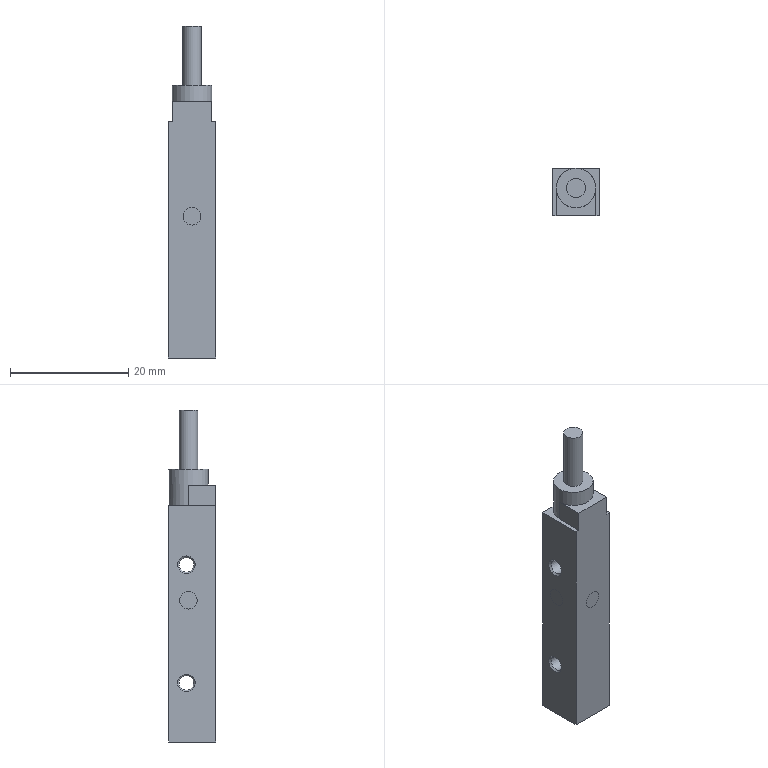Part | NX | features BREP 1 | 1 solid | 34 faces | box 8 x 8.1 x 56.2 mm | volume 2831 mm3 | plane 19 | cylinder 11 | cone 4 | commonest cylinder face diameters 3 x4 2.459 x2 3.2 x2 5.8 x1 6.7 x1 7 x1
STEP:
#1=CARTESIAN_POINT('',(0.,-4.65,-21.));
#2=VERTEX_POINT('',#1);
#3=CARTESIAN_POINT('',(0.,-4.65,-19.5));
#4=DIRECTION('',(0.,1.,0.));
#5=DIRECTION('',(0.,0.,-1.));
#6=AXIS2_PLACEMENT_3D('',#3,#4,#5);
#7=CIRCLE('',#6,1.5);
#8=EDGE_CURVE('',#2,#2,#7,.T.);
#9=ORIENTED_EDGE('',*,*,#8,.F.);
#10=EDGE_LOOP('',(#9));
#11=FACE_BOUND('',#10,.T.);
#12=CARTESIAN_POINT('',(0.,-4.649,-18.));
#13=VERTEX_POINT('',#12);
#14=CARTESIAN_POINT('',(0.,-4.649,-19.5));
#15=DIRECTION('',(0.,1.,0.));
#16=DIRECTION('',(0.,0.,1.));
#17=AXIS2_PLACEMENT_3D('',#14,#15,#16);
#18=CIRCLE('',#17,1.5);
#19=EDGE_CURVE('',#13,#13,#18,.T.);
#20=ORIENTED_EDGE('',*,*,#19,.T.);
#21=EDGE_LOOP('',(#20));
#22=FACE_BOUND('',#21,.T.);
#23=CARTESIAN_POINT('',(0.,5.,-19.5));
#24=DIRECTION('',(0.,-1.,0.));
#25=DIRECTION('',(0.,0.,1.));
#26=AXIS2_PLACEMENT_3D('',#23,#24,#25);
#27=CYLINDRICAL_SURFACE('',#26,1.5);
#28=ADVANCED_FACE('',(#11,#22),#27,.F.);
#29=CARTESIAN_POINT('',(-4.,0.,-18.));
#30=VERTEX_POINT('',#29);
#31=CARTESIAN_POINT('',(-4.,0.,-19.5));
#32=DIRECTION('',(1.,0.,0.));
#33=DIRECTION('',(0.,0.,1.));
#34=AXIS2_PLACEMENT_3D('',#31,#32,#33);
#35=CIRCLE('',#34,1.5);
#36=EDGE_CURVE('',#30,#30,#35,.T.);
#37=ORIENTED_EDGE('',*,*,#36,.F.);
#38=EDGE_LOOP('',(#37));
#39=FACE_BOUND('',#38,.T.);
#40=CARTESIAN_POINT('',(-3.999,0.,-21.));
#41=VERTEX_POINT('',#40);
#42=CARTESIAN_POINT('',(-3.999,0.,-19.5));
#43=DIRECTION('',(1.,0.,0.));
#44=DIRECTION('',(0.,0.,-1.));
#45=AXIS2_PLACEMENT_3D('',#42,#43,#44);
#46=CIRCLE('',#45,1.5);
#47=EDGE_CURVE('',#41,#41,#46,.T.);
#48=ORIENTED_EDGE('',*,*,#47,.T.);
#49=EDGE_LOOP('',(#48));
#50=FACE_BOUND('',#49,.T.);
#51=CARTESIAN_POINT('',(5.,0.,-19.5));
#52=DIRECTION('',(-1.,0.,0.));
#53=DIRECTION('',(0.,0.,-1.));
#54=AXIS2_PLACEMENT_3D('',#51,#52,#53);
#55=CYLINDRICAL_SURFACE('',#54,1.5);
#56=ADVANCED_FACE('',(#39,#50),#55,.F.);
#57=CARTESIAN_POINT('',(0.,3.349,-18.));
#58=VERTEX_POINT('',#57);
#59=CARTESIAN_POINT('',(0.,3.349,-19.5));
#60=DIRECTION('',(0.,1.,0.));
#61=DIRECTION('',(0.,0.,1.));
#62=AXIS2_PLACEMENT_3D('',#59,#60,#61);
#63=CIRCLE('',#62,1.5);
#64=EDGE_CURVE('',#58,#58,#63,.T.);
#65=ORIENTED_EDGE('',*,*,#64,.F.);
#66=EDGE_LOOP('',(#65));
#67=FACE_BOUND('',#66,.T.);
#68=CARTESIAN_POINT('',(0.,3.35,-18.));
#69=VERTEX_POINT('',#68);
#70=CARTESIAN_POINT('',(0.,3.35,-19.5));
#71=DIRECTION('',(0.,-1.,0.));
#72=DIRECTION('',(0.,0.,1.));
#73=AXIS2_PLACEMENT_3D('',#70,#71,#72);
#74=CIRCLE('',#73,1.5);
#75=EDGE_CURVE('',#69,#69,#74,.T.);
#76=ORIENTED_EDGE('',*,*,#75,.F.);
#77=EDGE_LOOP('',(#76));
#78=FACE_BOUND('',#77,.T.);
#79=CARTESIAN_POINT('',(0.,5.,-19.5));
#80=DIRECTION('',(0.,-1.,0.));
#81=DIRECTION('',(0.,0.,1.));
#82=AXIS2_PLACEMENT_3D('',#79,#80,#81);
#83=CYLINDRICAL_SURFACE('',#82,1.5);
#84=ADVANCED_FACE('',(#67,#78),#83,.F.);
#85=CARTESIAN_POINT('',(3.999,0.,-21.));
#86=VERTEX_POINT('',#85);
#87=CARTESIAN_POINT('',(3.999,0.,-19.5));
#88=DIRECTION('',(1.,0.,0.));
#89=DIRECTION('',(0.,0.,-1.));
#90=AXIS2_PLACEMENT_3D('',#87,#88,#89);
#91=CIRCLE('',#90,1.5);
#92=EDGE_CURVE('',#86,#86,#91,.T.);
#93=ORIENTED_EDGE('',*,*,#92,.F.);
#94=EDGE_LOOP('',(#93));
#95=FACE_BOUND('',#94,.T.);
#96=CARTESIAN_POINT('',(4.,0.,-21.));
#97=VERTEX_POINT('',#96);
#98=CARTESIAN_POINT('',(4.,0.,-19.5));
#99=DIRECTION('',(-1.,0.,0.));
#100=DIRECTION('',(0.,0.,-1.));
#101=AXIS2_PLACEMENT_3D('',#98,#99,#100);
#102=CIRCLE('',#101,1.5);
#103=EDGE_CURVE('',#97,#97,#102,.T.);
#104=ORIENTED_EDGE('',*,*,#103,.F.);
#105=EDGE_LOOP('',(#104));
#106=FACE_BOUND('',#105,.T.);
#107=CARTESIAN_POINT('',(5.,0.,-19.5));
#108=DIRECTION('',(-1.,0.,0.));
#109=DIRECTION('',(0.,0.,-1.));
#110=AXIS2_PLACEMENT_3D('',#107,#108,#109);
#111=CYLINDRICAL_SURFACE('',#110,1.5);
#112=ADVANCED_FACE('',(#95,#106),#111,.F.);
#113=CARTESIAN_POINT('',(3.35,0.,2.7));
#114=VERTEX_POINT('',#113);
#115=CARTESIAN_POINT('',(0.,0.,2.7));
#116=DIRECTION('',(0.,0.,1.));
#117=DIRECTION('',(1.,0.,0.));
#118=AXIS2_PLACEMENT_3D('',#115,#116,#117);
#119=CIRCLE('',#118,3.35);
#120=EDGE_CURVE('',#114,#114,#119,.T.);
#121=ORIENTED_EDGE('',*,*,#120,.F.);
#122=EDGE_LOOP('',(#121));
#123=FACE_BOUND('',#122,.T.);
#124=CARTESIAN_POINT('',(-3.35,0.,0.));
#125=VERTEX_POINT('',#124);
#126=CARTESIAN_POINT('',(3.35,0.,0.));
#127=VERTEX_POINT('',#126);
#128=CARTESIAN_POINT('',(0.,0.,0.));
#129=DIRECTION('',(0.,0.,1.));
#130=DIRECTION('',(1.,0.,0.));
#131=AXIS2_PLACEMENT_3D('',#128,#129,#130);
#132=CIRCLE('',#131,3.35);
#133=EDGE_CURVE('',#125,#127,#132,.T.);
#134=ORIENTED_EDGE('',*,*,#133,.T.);
#135=CARTESIAN_POINT('',(3.35,0.,-3.5));
#136=VERTEX_POINT('',#135);
#137=CARTESIAN_POINT('',(3.35,0.,-3.5));
#138=DIRECTION('',(0.,0.,1.));
#139=VECTOR('',#138,1000.);
#140=LINE('',#137,#139);
#141=EDGE_CURVE('',#136,#127,#140,.T.);
#142=ORIENTED_EDGE('',*,*,#141,.F.);
#143=CARTESIAN_POINT('',(0.,3.35,-3.5));
#144=VERTEX_POINT('',#143);
#145=CARTESIAN_POINT('',(0.,0.,-3.5));
#146=DIRECTION('',(0.,0.,1.));
#147=DIRECTION('',(1.,0.,0.));
#148=AXIS2_PLACEMENT_3D('',#145,#146,#147);
#149=CIRCLE('',#148,3.35);
#150=EDGE_CURVE('',#136,#144,#149,.T.);
#151=ORIENTED_EDGE('',*,*,#150,.T.);
#152=CARTESIAN_POINT('',(-3.35,0.,-3.5));
#153=VERTEX_POINT('',#152);
#154=CARTESIAN_POINT('',(0.,0.,-3.5));
#155=DIRECTION('',(0.,0.,1.));
#156=DIRECTION('',(1.,0.,0.));
#157=AXIS2_PLACEMENT_3D('',#154,#155,#156);
#158=CIRCLE('',#157,3.35);
#159=EDGE_CURVE('',#144,#153,#158,.T.);
#160=ORIENTED_EDGE('',*,*,#159,.T.);
#161=CARTESIAN_POINT('',(-3.35,0.,-3.5));
#162=DIRECTION('',(0.,0.,1.));
#163=VECTOR('',#162,1000.);
#164=LINE('',#161,#163);
#165=EDGE_CURVE('',#153,#125,#164,.T.);
#166=ORIENTED_EDGE('',*,*,#165,.T.);
#167=EDGE_LOOP('',(#134,#142,#151,#160,#166));
#168=FACE_BOUND('',#167,.T.);
#169=CARTESIAN_POINT('',(0.,0.,2.7));
#170=DIRECTION('',(0.,0.,-1.));
#171=DIRECTION('',(1.,0.,0.));
#172=AXIS2_PLACEMENT_3D('',#169,#170,#171);
#173=CYLINDRICAL_SURFACE('',#172,3.35);
#174=ADVANCED_FACE('',(#123,#168),#173,.T.);
#175=CARTESIAN_POINT('',(1.6,0.,2.7));
#176=VERTEX_POINT('',#175);
#177=CARTESIAN_POINT('',(0.,0.,2.7));
#178=DIRECTION('',(0.,0.,-1.));
#179=DIRECTION('',(1.,0.,0.));
#180=AXIS2_PLACEMENT_3D('',#177,#178,#179);
#181=CIRCLE('',#180,1.6);
#182=EDGE_CURVE('',#176,#176,#181,.T.);
#183=ORIENTED_EDGE('',*,*,#182,.T.);
#184=EDGE_LOOP('',(#183));
#185=FACE_BOUND('',#184,.T.);
#186=ORIENTED_EDGE('',*,*,#120,.T.);
#187=EDGE_LOOP('',(#186));
#188=FACE_BOUND('',#187,.T.);
#189=CARTESIAN_POINT('',(0.,0.,2.7));
#190=DIRECTION('',(0.,0.,1.));
#191=DIRECTION('',(-1.,0.,0.));
#192=AXIS2_PLACEMENT_3D('',#189,#190,#191);
#193=PLANE('',#192);
#194=ADVANCED_FACE('',(#185,#188),#193,.T.);
#195=ORIENTED_EDGE('',*,*,#133,.F.);
#196=CARTESIAN_POINT('',(-3.35,-4.65,0.));
#197=VERTEX_POINT('',#196);
#198=CARTESIAN_POINT('',(-3.35,0.,0.));
#199=DIRECTION('',(0.,-1.,0.));
#200=VECTOR('',#199,1000.);
#201=LINE('',#198,#200);
#202=EDGE_CURVE('',#125,#197,#201,.T.);
#203=ORIENTED_EDGE('',*,*,#202,.T.);
#204=CARTESIAN_POINT('',(3.35,-4.65,0.));
#205=VERTEX_POINT('',#204);
#206=CARTESIAN_POINT('',(-3.35,-4.65,0.));
#207=DIRECTION('',(1.,0.,0.));
#208=VECTOR('',#207,1000.);
#209=LINE('',#206,#208);
#210=EDGE_CURVE('',#197,#205,#209,.T.);
#211=ORIENTED_EDGE('',*,*,#210,.T.);
#212=CARTESIAN_POINT('',(3.35,-4.65,0.));
#213=DIRECTION('',(0.,1.,0.));
#214=VECTOR('',#213,1000.);
#215=LINE('',#212,#214);
#216=EDGE_CURVE('',#205,#127,#215,.T.);
#217=ORIENTED_EDGE('',*,*,#216,.T.);
#218=EDGE_LOOP('',(#195,#203,#211,#217));
#219=FACE_BOUND('',#218,.T.);
#220=CARTESIAN_POINT('',(0.,0.,0.));
#221=DIRECTION('',(0.,0.,1.));
#222=DIRECTION('',(-1.,0.,0.));
#223=AXIS2_PLACEMENT_3D('',#220,#221,#222);
#224=PLANE('',#223);
#225=ADVANCED_FACE('',(#219),#224,.T.);
#226=ORIENTED_EDGE('',*,*,#202,.F.);
#227=ORIENTED_EDGE('',*,*,#165,.F.);
#228=CARTESIAN_POINT('',(-3.35,-4.65,-3.5));
#229=VERTEX_POINT('',#228);
#230=CARTESIAN_POINT('',(-3.35,0.,-3.5));
#231=DIRECTION('',(0.,-1.,0.));
#232=VECTOR('',#231,1000.);
#233=LINE('',#230,#232);
#234=EDGE_CURVE('',#153,#229,#233,.T.);
#235=ORIENTED_EDGE('',*,*,#234,.T.);
#236=CARTESIAN_POINT('',(-3.35,-4.65,-3.5));
#237=DIRECTION('',(0.,0.,1.));
#238=VECTOR('',#237,1000.);
#239=LINE('',#236,#238);
#240=EDGE_CURVE('',#229,#197,#239,.T.);
#241=ORIENTED_EDGE('',*,*,#240,.T.);
#242=EDGE_LOOP('',(#226,#227,#235,#241));
#243=FACE_BOUND('',#242,.T.);
#244=CARTESIAN_POINT('',(-3.35,0.,-3.5));
#245=DIRECTION('',(-1.,0.,0.));
#246=DIRECTION('',(0.,0.,-1.));
#247=AXIS2_PLACEMENT_3D('',#244,#245,#246);
#248=PLANE('',#247);
#249=ADVANCED_FACE('',(#243),#248,.T.);
#250=ORIENTED_EDGE('',*,*,#8,.T.);
#251=EDGE_LOOP('',(#250));
#252=FACE_BOUND('',#251,.T.);
#253=ORIENTED_EDGE('',*,*,#210,.F.);
#254=ORIENTED_EDGE('',*,*,#240,.F.);
#255=CARTESIAN_POINT('',(-4.,-4.65,-3.5));
#256=VERTEX_POINT('',#255);
#257=CARTESIAN_POINT('',(-4.,-4.65,-3.5));
#258=DIRECTION('',(1.,0.,0.));
#259=VECTOR('',#258,1000.);
#260=LINE('',#257,#259);
#261=EDGE_CURVE('',#256,#229,#260,.T.);
#262=ORIENTED_EDGE('',*,*,#261,.F.);
#263=CARTESIAN_POINT('',(-4.,-4.65,-43.5));
#264=VERTEX_POINT('',#263);
#265=CARTESIAN_POINT('',(-4.,-4.65,-43.5));
#266=DIRECTION('',(0.,0.,1.));
#267=VECTOR('',#266,1000.);
#268=LINE('',#265,#267);
#269=EDGE_CURVE('',#264,#256,#268,.T.);
#270=ORIENTED_EDGE('',*,*,#269,.F.);
#271=CARTESIAN_POINT('',(4.,-4.65,-43.5));
#272=VERTEX_POINT('',#271);
#273=CARTESIAN_POINT('',(-4.,-4.65,-43.5));
#274=DIRECTION('',(1.,0.,0.));
#275=VECTOR('',#274,1000.);
#276=LINE('',#273,#275);
#277=EDGE_CURVE('',#264,#272,#276,.T.);
#278=ORIENTED_EDGE('',*,*,#277,.T.);
#279=CARTESIAN_POINT('',(4.,-4.65,-3.5));
#280=VERTEX_POINT('',#279);
#281=CARTESIAN_POINT('',(4.,-4.65,-43.5));
#282=DIRECTION('',(0.,0.,1.));
#283=VECTOR('',#282,1000.);
#284=LINE('',#281,#283);
#285=EDGE_CURVE('',#272,#280,#284,.T.);
#286=ORIENTED_EDGE('',*,*,#285,.T.);
#287=CARTESIAN_POINT('',(3.35,-4.65,-3.5));
#288=VERTEX_POINT('',#287);
#289=CARTESIAN_POINT('',(-4.,-4.65,-3.5));
#290=DIRECTION('',(1.,0.,0.));
#291=VECTOR('',#290,1000.);
#292=LINE('',#289,#291);
#293=EDGE_CURVE('',#288,#280,#292,.T.);
#294=ORIENTED_EDGE('',*,*,#293,.F.);
#295=CARTESIAN_POINT('',(3.35,-4.65,-3.5));
#296=DIRECTION('',(0.,0.,1.));
#297=VECTOR('',#296,1000.);
#298=LINE('',#295,#297);
#299=EDGE_CURVE('',#288,#205,#298,.T.);
#300=ORIENTED_EDGE('',*,*,#299,.T.);
#301=EDGE_LOOP('',(#253,#254,#262,#270,#278,#286,#294,#300));
#302=FACE_BOUND('',#301,.T.);
#303=CARTESIAN_POINT('',(-3.35,-4.65,-3.5));
#304=DIRECTION('',(0.,-1.,0.));
#305=DIRECTION('',(0.,0.,1.));
#306=AXIS2_PLACEMENT_3D('',#303,#304,#305);
#307=PLANE('',#306);
#308=ADVANCED_FACE('',(#252,#302),#307,.T.);
#309=ORIENTED_EDGE('',*,*,#216,.F.);
#310=ORIENTED_EDGE('',*,*,#299,.F.);
#311=CARTESIAN_POINT('',(3.35,-4.65,-3.5));
#312=DIRECTION('',(0.,1.,0.));
#313=VECTOR('',#312,1000.);
#314=LINE('',#311,#313);
#315=EDGE_CURVE('',#288,#136,#314,.T.);
#316=ORIENTED_EDGE('',*,*,#315,.T.);
#317=ORIENTED_EDGE('',*,*,#141,.T.);
#318=EDGE_LOOP('',(#309,#310,#316,#317));
#319=FACE_BOUND('',#318,.T.);
#320=CARTESIAN_POINT('',(3.35,-4.65,-3.5));
#321=DIRECTION('',(1.,0.,0.));
#322=DIRECTION('',(0.,0.,1.));
#323=AXIS2_PLACEMENT_3D('',#320,#321,#322);
#324=PLANE('',#323);
#325=ADVANCED_FACE('',(#319),#324,.T.);
#326=ORIENTED_EDGE('',*,*,#315,.F.);
#327=ORIENTED_EDGE('',*,*,#293,.T.);
#328=CARTESIAN_POINT('',(4.,3.35,-3.5));
#329=VERTEX_POINT('',#328);
#330=CARTESIAN_POINT('',(4.,-4.65,-3.5));
#331=DIRECTION('',(0.,1.,0.));
#332=VECTOR('',#331,1000.);
#333=LINE('',#330,#332);
#334=EDGE_CURVE('',#280,#329,#333,.T.);
#335=ORIENTED_EDGE('',*,*,#334,.T.);
#336=CARTESIAN_POINT('',(4.,3.35,-3.5));
#337=DIRECTION('',(-1.,0.,0.));
#338=VECTOR('',#337,1000.);
#339=LINE('',#336,#338);
#340=EDGE_CURVE('',#329,#144,#339,.T.);
#341=ORIENTED_EDGE('',*,*,#340,.T.);
#342=ORIENTED_EDGE('',*,*,#150,.F.);
#343=EDGE_LOOP('',(#326,#327,#335,#341,#342));
#344=FACE_BOUND('',#343,.T.);
#345=CARTESIAN_POINT('',(0.,0.,-3.5));
#346=DIRECTION('',(0.,0.,1.));
#347=DIRECTION('',(-1.,0.,0.));
#348=AXIS2_PLACEMENT_3D('',#345,#346,#347);
#349=PLANE('',#348);
#350=ADVANCED_FACE('',(#344),#349,.T.);
#351=ORIENTED_EDGE('',*,*,#159,.F.);
#352=CARTESIAN_POINT('',(-4.,3.35,-3.5));
#353=VERTEX_POINT('',#352);
#354=CARTESIAN_POINT('',(4.,3.35,-3.5));
#355=DIRECTION('',(-1.,0.,0.));
#356=VECTOR('',#355,1000.);
#357=LINE('',#354,#356);
#358=EDGE_CURVE('',#144,#353,#357,.T.);
#359=ORIENTED_EDGE('',*,*,#358,.T.);
#360=CARTESIAN_POINT('',(-4.,3.35,-3.5));
#361=DIRECTION('',(0.,-1.,0.));
#362=VECTOR('',#361,1000.);
#363=LINE('',#360,#362);
#364=EDGE_CURVE('',#353,#256,#363,.T.);
#365=ORIENTED_EDGE('',*,*,#364,.T.);
#366=ORIENTED_EDGE('',*,*,#261,.T.);
#367=ORIENTED_EDGE('',*,*,#234,.F.);
#368=EDGE_LOOP('',(#351,#359,#365,#366,#367));
#369=FACE_BOUND('',#368,.T.);
#370=CARTESIAN_POINT('',(0.,0.,-3.5));
#371=DIRECTION('',(0.,0.,1.));
#372=DIRECTION('',(-1.,0.,0.));
#373=AXIS2_PLACEMENT_3D('',#370,#371,#372);
#374=PLANE('',#373);
#375=ADVANCED_FACE('',(#369),#374,.T.);
#376=ORIENTED_EDGE('',*,*,#75,.T.);
#377=EDGE_LOOP('',(#376));
#378=FACE_BOUND('',#377,.T.);
#379=CARTESIAN_POINT('',(3.5,3.35,-38.5));
#380=VERTEX_POINT('',#379);
#381=CARTESIAN_POINT('',(0.,3.35,-38.5));
#382=DIRECTION('',(0.,1.,0.));
#383=DIRECTION('',(1.,0.,0.));
#384=AXIS2_PLACEMENT_3D('',#381,#382,#383);
#385=CIRCLE('',#384,3.5);
#386=EDGE_CURVE('',#380,#380,#385,.T.);
#387=ORIENTED_EDGE('',*,*,#386,.F.);
#388=EDGE_LOOP('',(#387));
#389=FACE_BOUND('',#388,.T.);
#390=ORIENTED_EDGE('',*,*,#340,.F.);
#391=CARTESIAN_POINT('',(4.,3.35,-43.5));
#392=VERTEX_POINT('',#391);
#393=CARTESIAN_POINT('',(4.,3.35,-43.5));
#394=DIRECTION('',(0.,0.,1.));
#395=VECTOR('',#394,1000.);
#396=LINE('',#393,#395);
#397=EDGE_CURVE('',#392,#329,#396,.T.);
#398=ORIENTED_EDGE('',*,*,#397,.F.);
#399=CARTESIAN_POINT('',(-4.,3.35,-43.5));
#400=VERTEX_POINT('',#399);
#401=CARTESIAN_POINT('',(4.,3.35,-43.5));
#402=DIRECTION('',(-1.,0.,0.));
#403=VECTOR('',#402,1000.);
#404=LINE('',#401,#403);
#405=EDGE_CURVE('',#392,#400,#404,.T.);
#406=ORIENTED_EDGE('',*,*,#405,.T.);
#407=CARTESIAN_POINT('',(-4.,3.35,-43.5));
#408=DIRECTION('',(0.,0.,1.));
#409=VECTOR('',#408,1000.);
#410=LINE('',#407,#409);
#411=EDGE_CURVE('',#400,#353,#410,.T.);
#412=ORIENTED_EDGE('',*,*,#411,.T.);
#413=ORIENTED_EDGE('',*,*,#358,.F.);
#414=EDGE_LOOP('',(#390,#398,#406,#412,#413));
#415=FACE_BOUND('',#414,.T.);
#416=CARTESIAN_POINT('',(4.,3.35,-43.5));
#417=DIRECTION('',(0.,1.,0.));
#418=DIRECTION('',(0.,0.,-1.));
#419=AXIS2_PLACEMENT_3D('',#416,#417,#418);
#420=PLANE('',#419);
#421=ADVANCED_FACE('',(#378,#389,#415),#420,.T.);
#422=ORIENTED_EDGE('',*,*,#36,.T.);
#423=EDGE_LOOP('',(#422));
#424=FACE_BOUND('',#423,.T.);
#425=CARTESIAN_POINT('',(-4.,0.35,-15.));
#426=VERTEX_POINT('',#425);
#427=CARTESIAN_POINT('',(-4.,0.35,-13.5));
#428=DIRECTION('',(1.,0.,0.));
#429=DIRECTION('',(0.,0.,-1.));
#430=AXIS2_PLACEMENT_3D('',#427,#428,#429);
#431=CIRCLE('',#430,1.5);
#432=EDGE_CURVE('',#426,#426,#431,.T.);
#433=ORIENTED_EDGE('',*,*,#432,.T.);
#434=EDGE_LOOP('',(#433));
#435=FACE_BOUND('',#434,.T.);
#436=CARTESIAN_POINT('',(-4.,0.35,-35.));
#437=VERTEX_POINT('',#436);
#438=CARTESIAN_POINT('',(-4.,0.35,-33.5));
#439=DIRECTION('',(1.,0.,0.));
#440=DIRECTION('',(0.,0.,-1.));
#441=AXIS2_PLACEMENT_3D('',#438,#439,#440);
#442=CIRCLE('',#441,1.5);
#443=EDGE_CURVE('',#437,#437,#442,.T.);
#444=ORIENTED_EDGE('',*,*,#443,.T.);
#445=EDGE_LOOP('',(#444));
#446=FACE_BOUND('',#445,.T.);
#447=ORIENTED_EDGE('',*,*,#364,.F.);
#448=ORIENTED_EDGE('',*,*,#411,.F.);
#449=CARTESIAN_POINT('',(-4.,3.35,-43.5));
#450=DIRECTION('',(0.,-1.,0.));
#451=VECTOR('',#450,1000.);
#452=LINE('',#449,#451);
#453=EDGE_CURVE('',#400,#264,#452,.T.);
#454=ORIENTED_EDGE('',*,*,#453,.T.);
#455=ORIENTED_EDGE('',*,*,#269,.T.);
#456=EDGE_LOOP('',(#447,#448,#454,#455));
#457=FACE_BOUND('',#456,.T.);
#458=CARTESIAN_POINT('',(-4.,3.35,-43.5));
#459=DIRECTION('',(-1.,0.,0.));
#460=DIRECTION('',(0.,0.,-1.));
#461=AXIS2_PLACEMENT_3D('',#458,#459,#460);
#462=PLANE('',#461);
#463=ADVANCED_FACE('',(#424,#435,#446,#457),#462,.T.);
#464=ORIENTED_EDGE('',*,*,#103,.T.);
#465=EDGE_LOOP('',(#464));
#466=FACE_BOUND('',#465,.T.);
#467=CARTESIAN_POINT('',(4.,0.35,-15.));
#468=VERTEX_POINT('',#467);
#469=CARTESIAN_POINT('',(4.,0.35,-13.5));
#470=DIRECTION('',(1.,0.,0.));
#471=DIRECTION('',(0.,0.,-1.));
#472=AXIS2_PLACEMENT_3D('',#469,#470,#471);
#473=CIRCLE('',#472,1.5);
#474=EDGE_CURVE('',#468,#468,#473,.T.);
#475=ORIENTED_EDGE('',*,*,#474,.F.);
#476=EDGE_LOOP('',(#475));
#477=FACE_BOUND('',#476,.T.);
#478=CARTESIAN_POINT('',(4.,0.35,-35.));
#479=VERTEX_POINT('',#478);
#480=CARTESIAN_POINT('',(4.,0.35,-33.5));
#481=DIRECTION('',(1.,0.,0.));
#482=DIRECTION('',(0.,0.,-1.));
#483=AXIS2_PLACEMENT_3D('',#480,#481,#482);
#484=CIRCLE('',#483,1.5);
#485=EDGE_CURVE('',#479,#479,#484,.T.);
#486=ORIENTED_EDGE('',*,*,#485,.F.);
#487=EDGE_LOOP('',(#486));
#488=FACE_BOUND('',#487,.T.);
#489=ORIENTED_EDGE('',*,*,#334,.F.);
#490=ORIENTED_EDGE('',*,*,#285,.F.);
#491=CARTESIAN_POINT('',(4.,-4.65,-43.5));
#492=DIRECTION('',(0.,1.,0.));
#493=VECTOR('',#492,1000.);
#494=LINE('',#491,#493);
#495=EDGE_CURVE('',#272,#392,#494,.T.);
#496=ORIENTED_EDGE('',*,*,#495,.T.);
#497=ORIENTED_EDGE('',*,*,#397,.T.);
#498=EDGE_LOOP('',(#489,#490,#496,#497));
#499=FACE_BOUND('',#498,.T.);
#500=CARTESIAN_POINT('',(4.,-4.65,-43.5));
#501=DIRECTION('',(1.,0.,0.));
#502=DIRECTION('',(0.,0.,1.));
#503=AXIS2_PLACEMENT_3D('',#500,#501,#502);
#504=PLANE('',#503);
#505=ADVANCED_FACE('',(#466,#477,#488,#499),#504,.T.);
#506=ORIENTED_EDGE('',*,*,#405,.F.);
#507=ORIENTED_EDGE('',*,*,#495,.F.);
#508=ORIENTED_EDGE('',*,*,#277,.F.);
#509=ORIENTED_EDGE('',*,*,#453,.F.);
#510=EDGE_LOOP('',(#506,#507,#508,#509));
#511=FACE_BOUND('',#510,.T.);
#512=CARTESIAN_POINT('',(0.,0.,-43.5));
#513=DIRECTION('',(0.,0.,1.));
#514=DIRECTION('',(-1.,0.,0.));
#515=AXIS2_PLACEMENT_3D('',#512,#513,#514);
#516=PLANE('',#515);
#517=ADVANCED_FACE('',(#511),#516,.F.);
#518=CARTESIAN_POINT('',(-3.729,0.35,-34.73));
#519=VERTEX_POINT('',#518);
#520=CARTESIAN_POINT('',(-3.729,0.35,-33.5));
#521=DIRECTION('',(1.,0.,0.));
#522=DIRECTION('',(0.,0.,-1.));
#523=AXIS2_PLACEMENT_3D('',#520,#521,#522);
#524=CIRCLE('',#523,1.23);
#525=EDGE_CURVE('',#519,#519,#524,.T.);
#526=ORIENTED_EDGE('',*,*,#525,.T.);
#527=EDGE_LOOP('',(#526));
#528=FACE_BOUND('',#527,.T.);
#529=ORIENTED_EDGE('',*,*,#443,.F.);
#530=EDGE_LOOP('',(#529));
#531=FACE_BOUND('',#530,.T.);
#532=CARTESIAN_POINT('',(-4.,0.35,-33.5));
#533=DIRECTION('',(-1.,0.,0.));
#534=DIRECTION('',(0.,0.,-1.));
#535=AXIS2_PLACEMENT_3D('',#532,#533,#534);
#536=CONICAL_SURFACE('',#535,1.5,0.7854);
#537=ADVANCED_FACE('',(#528,#531),#536,.F.);
#538=CARTESIAN_POINT('',(3.729,0.35,-34.73));
#539=VERTEX_POINT('',#538);
#540=CARTESIAN_POINT('',(3.729,0.35,-33.5));
#541=DIRECTION('',(1.,0.,0.));
#542=DIRECTION('',(0.,0.,-1.));
#543=AXIS2_PLACEMENT_3D('',#540,#541,#542);
#544=CIRCLE('',#543,1.23);
#545=EDGE_CURVE('',#539,#539,#544,.T.);
#546=ORIENTED_EDGE('',*,*,#545,.T.);
#547=EDGE_LOOP('',(#546));
#548=FACE_BOUND('',#547,.T.);
#549=ORIENTED_EDGE('',*,*,#525,.F.);
#550=EDGE_LOOP('',(#549));
#551=FACE_BOUND('',#550,.T.);
#552=CARTESIAN_POINT('',(4.,0.35,-33.5));
#553=DIRECTION('',(1.,0.,0.));
#554=DIRECTION('',(0.,0.,1.));
#555=AXIS2_PLACEMENT_3D('',#552,#553,#554);
#556=CYLINDRICAL_SURFACE('',#555,1.23);
#557=ADVANCED_FACE('',(#548,#551),#556,.F.);
#558=ORIENTED_EDGE('',*,*,#485,.T.);
#559=EDGE_LOOP('',(#558));
#560=FACE_BOUND('',#559,.T.);
#561=ORIENTED_EDGE('',*,*,#545,.F.);
#562=EDGE_LOOP('',(#561));
#563=FACE_BOUND('',#562,.T.);
#564=CARTESIAN_POINT('',(3.729,0.35,-33.5));
#565=DIRECTION('',(1.,0.,0.));
#566=DIRECTION('',(0.,0.,1.));
#567=AXIS2_PLACEMENT_3D('',#564,#565,#566);
#568=CONICAL_SURFACE('',#567,1.23,0.7854);
#569=ADVANCED_FACE('',(#560,#563),#568,.F.);
#570=CARTESIAN_POINT('',(-3.729,0.35,-14.729));
#571=VERTEX_POINT('',#570);
#572=CARTESIAN_POINT('',(-3.729,0.35,-13.5));
#573=DIRECTION('',(1.,0.,0.));
#574=DIRECTION('',(0.,0.,-1.));
#575=AXIS2_PLACEMENT_3D('',#572,#573,#574);
#576=CIRCLE('',#575,1.23);
#577=EDGE_CURVE('',#571,#571,#576,.T.);
#578=ORIENTED_EDGE('',*,*,#577,.T.);
#579=EDGE_LOOP('',(#578));
#580=FACE_BOUND('',#579,.T.);
#581=ORIENTED_EDGE('',*,*,#432,.F.);
#582=EDGE_LOOP('',(#581));
#583=FACE_BOUND('',#582,.T.);
#584=CARTESIAN_POINT('',(-4.,0.35,-13.5));
#585=DIRECTION('',(-1.,0.,0.));
#586=DIRECTION('',(0.,0.,-1.));
#587=AXIS2_PLACEMENT_3D('',#584,#585,#586);
#588=CONICAL_SURFACE('',#587,1.5,0.7854);
#589=ADVANCED_FACE('',(#580,#583),#588,.F.);
#590=CARTESIAN_POINT('',(3.729,0.35,-14.729));
#591=VERTEX_POINT('',#590);
#592=CARTESIAN_POINT('',(3.729,0.35,-13.5));
#593=DIRECTION('',(1.,0.,0.));
#594=DIRECTION('',(0.,0.,-1.));
#595=AXIS2_PLACEMENT_3D('',#592,#593,#594);
#596=CIRCLE('',#595,1.23);
#597=EDGE_CURVE('',#591,#591,#596,.T.);
#598=ORIENTED_EDGE('',*,*,#597,.T.);
#599=EDGE_LOOP('',(#598));
#600=FACE_BOUND('',#599,.T.);
#601=ORIENTED_EDGE('',*,*,#577,.F.);
#602=EDGE_LOOP('',(#601));
#603=FACE_BOUND('',#602,.T.);
#604=CARTESIAN_POINT('',(4.,0.35,-13.5));
#605=DIRECTION('',(1.,0.,0.));
#606=DIRECTION('',(0.,0.,1.));
#607=AXIS2_PLACEMENT_3D('',#604,#605,#606);
#608=CYLINDRICAL_SURFACE('',#607,1.23);
#609=ADVANCED_FACE('',(#600,#603),#608,.F.);
#610=ORIENTED_EDGE('',*,*,#474,.T.);
#611=EDGE_LOOP('',(#610));
#612=FACE_BOUND('',#611,.T.);
#613=ORIENTED_EDGE('',*,*,#597,.F.);
#614=EDGE_LOOP('',(#613));
#615=FACE_BOUND('',#614,.T.);
#616=CARTESIAN_POINT('',(3.729,0.35,-13.5));
#617=DIRECTION('',(1.,0.,0.));
#618=DIRECTION('',(0.,0.,1.));
#619=AXIS2_PLACEMENT_3D('',#616,#617,#618);
#620=CONICAL_SURFACE('',#619,1.23,0.7854);
#621=ADVANCED_FACE('',(#612,#615),#620,.F.);
#622=CARTESIAN_POINT('',(2.9,3.45,-38.5));
#623=VERTEX_POINT('',#622);
#624=CARTESIAN_POINT('',(0.,3.45,-38.5));
#625=DIRECTION('',(0.,1.,0.));
#626=DIRECTION('',(1.,0.,0.));
#627=AXIS2_PLACEMENT_3D('',#624,#625,#626);
#628=CIRCLE('',#627,2.9);
#629=EDGE_CURVE('',#623,#623,#628,.T.);
#630=ORIENTED_EDGE('',*,*,#629,.T.);
#631=EDGE_LOOP('',(#630));
#632=FACE_BOUND('',#631,.T.);
#633=CARTESIAN_POINT('',(0.,3.35,-35.6));
#634=VERTEX_POINT('',#633);
#635=CARTESIAN_POINT('',(0.,3.35,-38.5));
#636=DIRECTION('',(0.,-1.,0.));
#637=DIRECTION('',(0.,0.,1.));
#638=AXIS2_PLACEMENT_3D('',#635,#636,#637);
#639=CIRCLE('',#638,2.9);
#640=EDGE_CURVE('',#634,#634,#639,.T.);
#641=ORIENTED_EDGE('',*,*,#640,.T.);
#642=EDGE_LOOP('',(#641));
#643=FACE_BOUND('',#642,.T.);
#644=CARTESIAN_POINT('',(0.,3.45,-38.5));
#645=DIRECTION('',(0.,-1.,0.));
#646=DIRECTION('',(0.,0.,1.));
#647=AXIS2_PLACEMENT_3D('',#644,#645,#646);
#648=CYLINDRICAL_SURFACE('',#647,2.9);
#649=ADVANCED_FACE('',(#632,#643),#648,.F.);
#650=CARTESIAN_POINT('',(3.5,3.45,-38.5));
#651=VERTEX_POINT('',#650);
#652=CARTESIAN_POINT('',(0.,3.45,-38.5));
#653=DIRECTION('',(0.,1.,0.));
#654=DIRECTION('',(1.,0.,0.));
#655=AXIS2_PLACEMENT_3D('',#652,#653,#654);
#656=CIRCLE('',#655,3.5);
#657=EDGE_CURVE('',#651,#651,#656,.T.);
#658=ORIENTED_EDGE('',*,*,#657,.F.);
#659=EDGE_LOOP('',(#658));
#660=FACE_BOUND('',#659,.T.);
#661=ORIENTED_EDGE('',*,*,#386,.T.);
#662=EDGE_LOOP('',(#661));
#663=FACE_BOUND('',#662,.T.);
#664=CARTESIAN_POINT('',(0.,3.45,-38.5));
#665=DIRECTION('',(0.,-1.,0.));
#666=DIRECTION('',(0.,0.,1.));
#667=AXIS2_PLACEMENT_3D('',#664,#665,#666);
#668=CYLINDRICAL_SURFACE('',#667,3.5);
#669=ADVANCED_FACE('',(#660,#663),#668,.T.);
#670=ORIENTED_EDGE('',*,*,#629,.F.);
#671=EDGE_LOOP('',(#670));
#672=FACE_BOUND('',#671,.T.);
#673=ORIENTED_EDGE('',*,*,#657,.T.);
#674=EDGE_LOOP('',(#673));
#675=FACE_BOUND('',#674,.T.);
#676=CARTESIAN_POINT('',(0.,3.45,-38.5));
#677=DIRECTION('',(0.,1.,0.));
#678=DIRECTION('',(0.,0.,-1.));
#679=AXIS2_PLACEMENT_3D('',#676,#677,#678);
#680=PLANE('',#679);
#681=ADVANCED_FACE('',(#672,#675),#680,.T.);
#682=CARTESIAN_POINT('',(1.6,3.35,-38.5));
#683=VERTEX_POINT('',#682);
#684=CARTESIAN_POINT('',(0.,3.35,-38.5));
#685=DIRECTION('',(0.,1.,0.));
#686=DIRECTION('',(1.,0.,0.));
#687=AXIS2_PLACEMENT_3D('',#684,#685,#686);
#688=CIRCLE('',#687,1.6);
#689=EDGE_CURVE('',#683,#683,#688,.T.);
#690=ORIENTED_EDGE('',*,*,#689,.F.);
#691=EDGE_LOOP('',(#690));
#692=FACE_BOUND('',#691,.T.);
#693=ORIENTED_EDGE('',*,*,#640,.F.);
#694=EDGE_LOOP('',(#693));
#695=FACE_BOUND('',#694,.T.);
#696=CARTESIAN_POINT('',(4.,3.35,-43.5));
#697=DIRECTION('',(0.,1.,0.));
#698=DIRECTION('',(0.,0.,-1.));
#699=AXIS2_PLACEMENT_3D('',#696,#697,#698);
#700=PLANE('',#699);
#701=ADVANCED_FACE('',(#692,#695),#700,.T.);
#702=CARTESIAN_POINT('',(1.6,3.45,-38.5));
#703=VERTEX_POINT('',#702);
#704=CARTESIAN_POINT('',(0.,3.45,-38.5));
#705=DIRECTION('',(0.,1.,0.));
#706=DIRECTION('',(1.,0.,0.));
#707=AXIS2_PLACEMENT_3D('',#704,#705,#706);
#708=CIRCLE('',#707,1.6);
#709=EDGE_CURVE('',#703,#703,#708,.T.);
#710=ORIENTED_EDGE('',*,*,#709,.F.);
#711=EDGE_LOOP('',(#710));
#712=FACE_BOUND('',#711,.T.);
#713=ORIENTED_EDGE('',*,*,#689,.T.);
#714=EDGE_LOOP('',(#713));
#715=FACE_BOUND('',#714,.T.);
#716=CARTESIAN_POINT('',(0.,3.45,-38.5));
#717=DIRECTION('',(0.,-1.,0.));
#718=DIRECTION('',(0.,0.,1.));
#719=AXIS2_PLACEMENT_3D('',#716,#717,#718);
#720=CYLINDRICAL_SURFACE('',#719,1.6);
#721=ADVANCED_FACE('',(#712,#715),#720,.T.);
#722=ORIENTED_EDGE('',*,*,#709,.T.);
#723=EDGE_LOOP('',(#722));
#724=FACE_BOUND('',#723,.T.);
#725=CARTESIAN_POINT('',(0.,3.45,-38.5));
#726=DIRECTION('',(0.,1.,0.));
#727=DIRECTION('',(0.,0.,-1.));
#728=AXIS2_PLACEMENT_3D('',#725,#726,#727);
#729=PLANE('',#728);
#730=ADVANCED_FACE('',(#724),#729,.T.);
#731=ORIENTED_EDGE('',*,*,#182,.F.);
#732=EDGE_LOOP('',(#731));
#733=FACE_BOUND('',#732,.T.);
#734=CARTESIAN_POINT('',(1.6,0.,12.7));
#735=VERTEX_POINT('',#734);
#736=CARTESIAN_POINT('',(0.,0.,12.7));
#737=DIRECTION('',(0.,0.,1.));
#738=DIRECTION('',(1.,0.,0.));
#739=AXIS2_PLACEMENT_3D('',#736,#737,#738);
#740=CIRCLE('',#739,1.6);
#741=EDGE_CURVE('',#735,#735,#740,.T.);
#742=ORIENTED_EDGE('',*,*,#741,.F.);
#743=EDGE_LOOP('',(#742));
#744=FACE_BOUND('',#743,.T.);
#745=CARTESIAN_POINT('',(0.,0.,12.7));
#746=DIRECTION('',(0.,0.,-1.));
#747=DIRECTION('',(1.,0.,0.));
#748=AXIS2_PLACEMENT_3D('',#745,#746,#747);
#749=CYLINDRICAL_SURFACE('',#748,1.6);
#750=ADVANCED_FACE('',(#733,#744),#749,.T.);
#751=ORIENTED_EDGE('',*,*,#741,.T.);
#752=EDGE_LOOP('',(#751));
#753=FACE_BOUND('',#752,.T.);
#754=CARTESIAN_POINT('',(0.,0.,12.7));
#755=DIRECTION('',(0.,0.,1.));
#756=DIRECTION('',(-1.,0.,0.));
#757=AXIS2_PLACEMENT_3D('',#754,#755,#756);
#758=PLANE('',#757);
#759=ADVANCED_FACE('',(#753),#758,.T.);
#760=ORIENTED_EDGE('',*,*,#92,.T.);
#761=EDGE_LOOP('',(#760));
#762=FACE_BOUND('',#761,.T.);
#763=CARTESIAN_POINT('',(3.999,0.,-19.5));
#764=DIRECTION('',(1.,0.,0.));
#765=DIRECTION('',(0.,0.,1.));
#766=AXIS2_PLACEMENT_3D('',#763,#764,#765);
#767=PLANE('',#766);
#768=ADVANCED_FACE('',(#762),#767,.T.);
#769=ORIENTED_EDGE('',*,*,#47,.F.);
#770=EDGE_LOOP('',(#769));
#771=FACE_BOUND('',#770,.T.);
#772=CARTESIAN_POINT('',(-3.999,0.,-19.5));
#773=DIRECTION('',(1.,0.,0.));
#774=DIRECTION('',(0.,0.,1.));
#775=AXIS2_PLACEMENT_3D('',#772,#773,#774);
#776=PLANE('',#775);
#777=ADVANCED_FACE('',(#771),#776,.F.);
#778=ORIENTED_EDGE('',*,*,#64,.T.);
#779=EDGE_LOOP('',(#778));
#780=FACE_BOUND('',#779,.T.);
#781=CARTESIAN_POINT('',(0.,3.349,-19.5));
#782=DIRECTION('',(0.,1.,0.));
#783=DIRECTION('',(0.,0.,-1.));
#784=AXIS2_PLACEMENT_3D('',#781,#782,#783);
#785=PLANE('',#784);
#786=ADVANCED_FACE('',(#780),#785,.T.);
#787=ORIENTED_EDGE('',*,*,#19,.F.);
#788=EDGE_LOOP('',(#787));
#789=FACE_BOUND('',#788,.T.);
#790=CARTESIAN_POINT('',(0.,-4.649,-19.5));
#791=DIRECTION('',(0.,1.,0.));
#792=DIRECTION('',(0.,0.,-1.));
#793=AXIS2_PLACEMENT_3D('',#790,#791,#792);
#794=PLANE('',#793);
#795=ADVANCED_FACE('',(#789),#794,.F.);
#796=CLOSED_SHELL('',(#28,#56,#84,#112,#174,#194,#225,#249,#308,#325,#350,#375,#421,#463,#505,#517,#537,#557,#569,#589,#609,#621,#649,#669,#681,#701,#721,#730,#750,#759,#768,#777,#786,#795));
#797=MANIFOLD_SOLID_BREP('',#796);
#798=(LENGTH_UNIT()NAMED_UNIT(*)SI_UNIT(.MILLI.,.METRE.));
#799=UNCERTAINTY_MEASURE_WITH_UNIT(LENGTH_MEASURE(0.00001),#798,'','');
#800=(NAMED_UNIT(*)PLANE_ANGLE_UNIT()SI_UNIT($,.RADIAN.));
#801=(NAMED_UNIT(*)SI_UNIT($,.STERADIAN.)SOLID_ANGLE_UNIT());
#802=(GEOMETRIC_REPRESENTATION_CONTEXT(3)GLOBAL_UNCERTAINTY_ASSIGNED_CONTEXT((#799))GLOBAL_UNIT_ASSIGNED_CONTEXT((#798,#800,#801))REPRESENTATION_CONTEXT('',''));
#803=ADVANCED_BREP_SHAPE_REPRESENTATION('',(#797),#802);